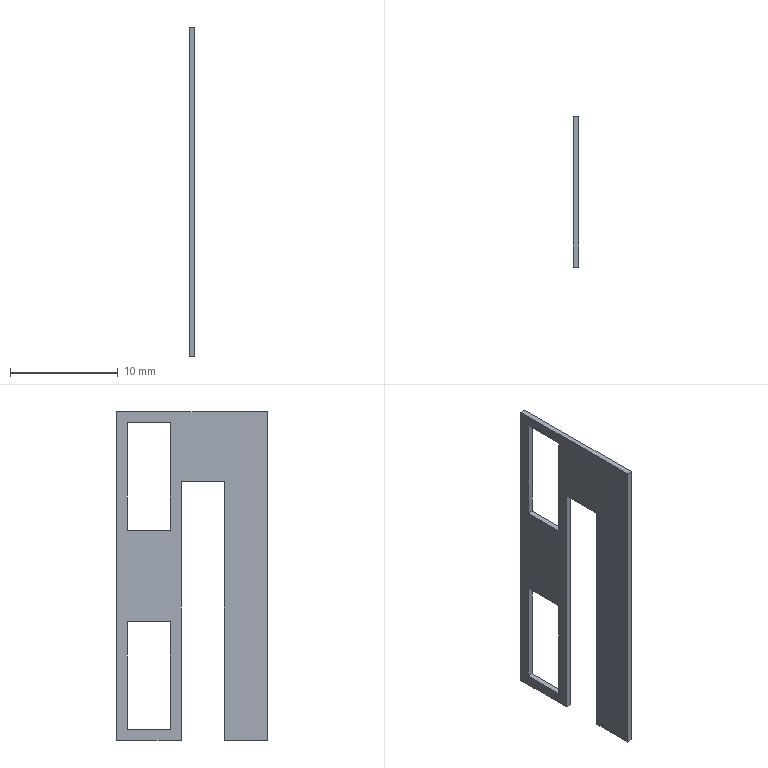Part | SolidWorks | features BaseBody 1 | 1 solid | 823 faces | box 0.5 x 14 x 30.5 mm | volume 122.527 mm3 | plane 636 | spline 187